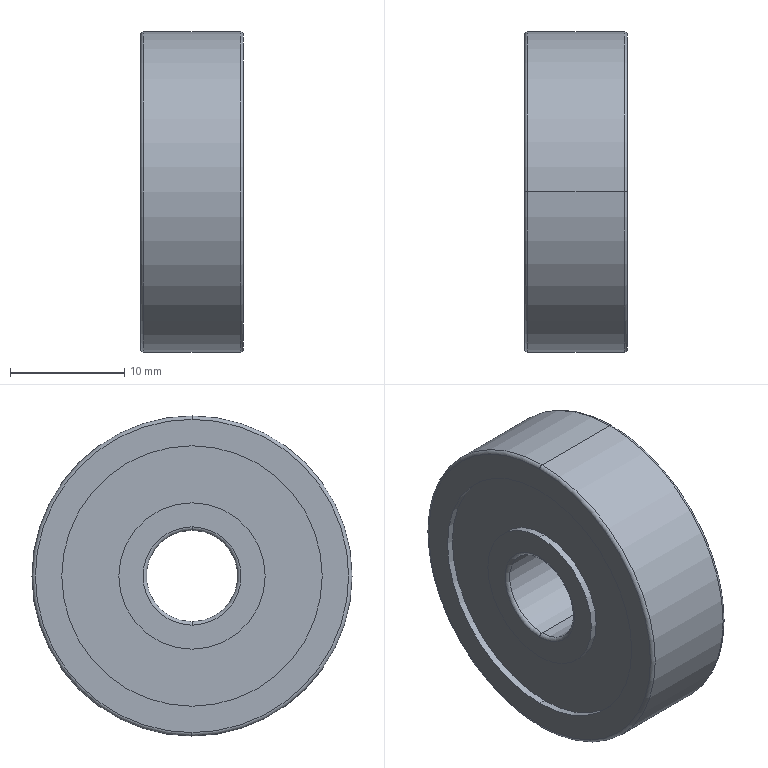Part | SolidWorks | features RefAxis 3, Revolution 1 | 1 solid | 26 faces | box 9 x 28 x 28 mm | volume 4750 mm3 | cylinder 12 | torus 8 | plane 6 | commonest cylinder face diameters 12.8 x4 22.78 x4 8 x2 28 x2
STEP:
#1=CARTESIAN_POINT('',(8.7,0.,-4.));
#2=VERTEX_POINT('',#1);
#3=CARTESIAN_POINT('',(8.7,0.,4.));
#4=VERTEX_POINT('',#3);
#5=CARTESIAN_POINT('',(8.7,0.,0.));
#6=DIRECTION('',(-1.,0.,0.));
#7=DIRECTION('',(0.,0.,1.));
#8=AXIS2_PLACEMENT_3D('',#5,#6,#7);
#9=CIRCLE('',#8,4.);
#10=EDGE_CURVE('',#2,#4,#9,.T.);
#11=ORIENTED_EDGE('',*,*,#10,.F.);
#12=CARTESIAN_POINT('',(0.3,0.,-4.));
#13=VERTEX_POINT('',#12);
#14=CARTESIAN_POINT('',(-0.115,0.,-4.));
#15=DIRECTION('',(-1.,0.,0.));
#16=VECTOR('',#15,1000.);
#17=LINE('',#14,#16);
#18=EDGE_CURVE('',#2,#13,#17,.T.);
#19=ORIENTED_EDGE('',*,*,#18,.T.);
#20=CARTESIAN_POINT('',(0.3,0.,4.));
#21=VERTEX_POINT('',#20);
#22=CARTESIAN_POINT('',(0.3,0.,0.));
#23=DIRECTION('',(-1.,0.,0.));
#24=DIRECTION('',(0.,0.,1.));
#25=AXIS2_PLACEMENT_3D('',#22,#23,#24);
#26=CIRCLE('',#25,4.);
#27=EDGE_CURVE('',#13,#21,#26,.T.);
#28=ORIENTED_EDGE('',*,*,#27,.T.);
#29=CARTESIAN_POINT('',(-0.115,0.,4.));
#30=DIRECTION('',(-1.,0.,0.));
#31=VECTOR('',#30,1000.);
#32=LINE('',#29,#31);
#33=EDGE_CURVE('',#4,#21,#32,.T.);
#34=ORIENTED_EDGE('',*,*,#33,.F.);
#35=EDGE_LOOP('',(#11,#19,#28,#34));
#36=FACE_OUTER_BOUND('',#35,.T.);
#37=CARTESIAN_POINT('',(-0.115,0.,0.));
#38=DIRECTION('',(-1.,0.,0.));
#39=DIRECTION('',(0.,0.,1.));
#40=AXIS2_PLACEMENT_3D('',#37,#38,#39);
#41=CYLINDRICAL_SURFACE('',#40,4.);
#42=ADVANCED_FACE('',(#36),#41,.F.);
#43=CARTESIAN_POINT('',(8.7,0.,0.));
#44=DIRECTION('',(-1.,0.,0.));
#45=DIRECTION('',(0.,0.,1.));
#46=AXIS2_PLACEMENT_3D('',#43,#44,#45);
#47=CIRCLE('',#46,4.);
#48=EDGE_CURVE('',#4,#2,#47,.T.);
#49=ORIENTED_EDGE('',*,*,#48,.T.);
#50=CARTESIAN_POINT('',(9.,0.,-4.3));
#51=VERTEX_POINT('',#50);
#52=CARTESIAN_POINT('',(8.7,0.,-4.3));
#53=DIRECTION('',(0.,1.,0.));
#54=DIRECTION('',(0.,0.,1.));
#55=AXIS2_PLACEMENT_3D('',#52,#53,#54);
#56=CIRCLE('',#55,0.3);
#57=EDGE_CURVE('',#2,#51,#56,.T.);
#58=ORIENTED_EDGE('',*,*,#57,.T.);
#59=CARTESIAN_POINT('',(9.,0.,4.3));
#60=VERTEX_POINT('',#59);
#61=CARTESIAN_POINT('',(9.,0.,0.));
#62=DIRECTION('',(-1.,0.,0.));
#63=DIRECTION('',(0.,0.,1.));
#64=AXIS2_PLACEMENT_3D('',#61,#62,#63);
#65=CIRCLE('',#64,4.3);
#66=EDGE_CURVE('',#60,#51,#65,.T.);
#67=ORIENTED_EDGE('',*,*,#66,.F.);
#68=CARTESIAN_POINT('',(8.7,0.,4.3));
#69=DIRECTION('',(0.,-1.,0.));
#70=DIRECTION('',(0.,0.,-1.));
#71=AXIS2_PLACEMENT_3D('',#68,#69,#70);
#72=CIRCLE('',#71,0.3);
#73=EDGE_CURVE('',#4,#60,#72,.T.);
#74=ORIENTED_EDGE('',*,*,#73,.F.);
#75=EDGE_LOOP('',(#49,#58,#67,#74));
#76=FACE_OUTER_BOUND('',#75,.T.);
#77=CARTESIAN_POINT('',(8.7,0.,0.));
#78=DIRECTION('',(-1.,0.,0.));
#79=DIRECTION('',(0.,0.,1.));
#80=AXIS2_PLACEMENT_3D('',#77,#78,#79);
#81=TOROIDAL_SURFACE('',#80,4.3,0.3);
#82=ADVANCED_FACE('',(#76),#81,.T.);
#83=CARTESIAN_POINT('',(9.,0.,6.4));
#84=VERTEX_POINT('',#83);
#85=CARTESIAN_POINT('',(9.,0.,-6.4));
#86=VERTEX_POINT('',#85);
#87=CARTESIAN_POINT('',(9.,0.,0.));
#88=DIRECTION('',(-1.,0.,0.));
#89=DIRECTION('',(0.,0.,1.));
#90=AXIS2_PLACEMENT_3D('',#87,#88,#89);
#91=CIRCLE('',#90,6.4);
#92=EDGE_CURVE('',#84,#86,#91,.T.);
#93=ORIENTED_EDGE('',*,*,#92,.T.);
#94=CARTESIAN_POINT('',(8.4,0.,-6.4));
#95=VERTEX_POINT('',#94);
#96=CARTESIAN_POINT('',(-0.115,0.,-6.4));
#97=DIRECTION('',(-1.,0.,0.));
#98=VECTOR('',#97,1000.);
#99=LINE('',#96,#98);
#100=EDGE_CURVE('',#86,#95,#99,.T.);
#101=ORIENTED_EDGE('',*,*,#100,.T.);
#102=CARTESIAN_POINT('',(8.4,0.,6.4));
#103=VERTEX_POINT('',#102);
#104=CARTESIAN_POINT('',(8.4,0.,0.));
#105=DIRECTION('',(-1.,0.,0.));
#106=DIRECTION('',(0.,0.,1.));
#107=AXIS2_PLACEMENT_3D('',#104,#105,#106);
#108=CIRCLE('',#107,6.4);
#109=EDGE_CURVE('',#103,#95,#108,.T.);
#110=ORIENTED_EDGE('',*,*,#109,.F.);
#111=CARTESIAN_POINT('',(-0.115,0.,6.4));
#112=DIRECTION('',(-1.,0.,0.));
#113=VECTOR('',#112,1000.);
#114=LINE('',#111,#113);
#115=EDGE_CURVE('',#84,#103,#114,.T.);
#116=ORIENTED_EDGE('',*,*,#115,.F.);
#117=EDGE_LOOP('',(#93,#101,#110,#116));
#118=FACE_OUTER_BOUND('',#117,.T.);
#119=CARTESIAN_POINT('',(-0.115,0.,0.));
#120=DIRECTION('',(-1.,0.,0.));
#121=DIRECTION('',(0.,0.,1.));
#122=AXIS2_PLACEMENT_3D('',#119,#120,#121);
#123=CYLINDRICAL_SURFACE('',#122,6.4);
#124=ADVANCED_FACE('',(#118),#123,.T.);
#125=CARTESIAN_POINT('',(9.,0.,-11.39));
#126=VERTEX_POINT('',#125);
#127=CARTESIAN_POINT('',(9.,0.,11.39));
#128=VERTEX_POINT('',#127);
#129=CARTESIAN_POINT('',(9.,0.,0.));
#130=DIRECTION('',(-1.,0.,0.));
#131=DIRECTION('',(0.,0.,1.));
#132=AXIS2_PLACEMENT_3D('',#129,#130,#131);
#133=CIRCLE('',#132,11.39);
#134=EDGE_CURVE('',#126,#128,#133,.T.);
#135=ORIENTED_EDGE('',*,*,#134,.F.);
#136=CARTESIAN_POINT('',(8.4,0.,-11.39));
#137=VERTEX_POINT('',#136);
#138=CARTESIAN_POINT('',(-0.115,0.,-11.39));
#139=DIRECTION('',(-1.,0.,0.));
#140=VECTOR('',#139,1000.);
#141=LINE('',#138,#140);
#142=EDGE_CURVE('',#126,#137,#141,.T.);
#143=ORIENTED_EDGE('',*,*,#142,.T.);
#144=CARTESIAN_POINT('',(8.4,0.,11.39));
#145=VERTEX_POINT('',#144);
#146=CARTESIAN_POINT('',(8.4,0.,0.));
#147=DIRECTION('',(-1.,0.,0.));
#148=DIRECTION('',(0.,0.,1.));
#149=AXIS2_PLACEMENT_3D('',#146,#147,#148);
#150=CIRCLE('',#149,11.39);
#151=EDGE_CURVE('',#137,#145,#150,.T.);
#152=ORIENTED_EDGE('',*,*,#151,.T.);
#153=CARTESIAN_POINT('',(-0.115,0.,11.39));
#154=DIRECTION('',(-1.,0.,0.));
#155=VECTOR('',#154,1000.);
#156=LINE('',#153,#155);
#157=EDGE_CURVE('',#128,#145,#156,.T.);
#158=ORIENTED_EDGE('',*,*,#157,.F.);
#159=EDGE_LOOP('',(#135,#143,#152,#158));
#160=FACE_OUTER_BOUND('',#159,.T.);
#161=CARTESIAN_POINT('',(-0.115,0.,0.));
#162=DIRECTION('',(-1.,0.,0.));
#163=DIRECTION('',(0.,0.,1.));
#164=AXIS2_PLACEMENT_3D('',#161,#162,#163);
#165=CYLINDRICAL_SURFACE('',#164,11.39);
#166=ADVANCED_FACE('',(#160),#165,.F.);
#167=CARTESIAN_POINT('',(9.,0.,13.7));
#168=VERTEX_POINT('',#167);
#169=CARTESIAN_POINT('',(9.,0.,-13.7));
#170=VERTEX_POINT('',#169);
#171=CARTESIAN_POINT('',(9.,0.,0.));
#172=DIRECTION('',(-1.,0.,0.));
#173=DIRECTION('',(0.,0.,1.));
#174=AXIS2_PLACEMENT_3D('',#171,#172,#173);
#175=CIRCLE('',#174,13.7);
#176=EDGE_CURVE('',#168,#170,#175,.T.);
#177=ORIENTED_EDGE('',*,*,#176,.T.);
#178=CARTESIAN_POINT('',(8.7,0.,-14.));
#179=VERTEX_POINT('',#178);
#180=CARTESIAN_POINT('',(8.7,0.,-13.7));
#181=DIRECTION('',(0.,1.,0.));
#182=DIRECTION('',(0.,0.,1.));
#183=AXIS2_PLACEMENT_3D('',#180,#181,#182);
#184=CIRCLE('',#183,0.3);
#185=EDGE_CURVE('',#170,#179,#184,.T.);
#186=ORIENTED_EDGE('',*,*,#185,.T.);
#187=CARTESIAN_POINT('',(8.7,0.,14.));
#188=VERTEX_POINT('',#187);
#189=CARTESIAN_POINT('',(8.7,0.,0.));
#190=DIRECTION('',(-1.,0.,0.));
#191=DIRECTION('',(0.,0.,1.));
#192=AXIS2_PLACEMENT_3D('',#189,#190,#191);
#193=CIRCLE('',#192,14.);
#194=EDGE_CURVE('',#188,#179,#193,.T.);
#195=ORIENTED_EDGE('',*,*,#194,.F.);
#196=CARTESIAN_POINT('',(8.7,0.,13.7));
#197=DIRECTION('',(0.,-1.,0.));
#198=DIRECTION('',(0.,0.,-1.));
#199=AXIS2_PLACEMENT_3D('',#196,#197,#198);
#200=CIRCLE('',#199,0.3);
#201=EDGE_CURVE('',#168,#188,#200,.T.);
#202=ORIENTED_EDGE('',*,*,#201,.F.);
#203=EDGE_LOOP('',(#177,#186,#195,#202));
#204=FACE_OUTER_BOUND('',#203,.T.);
#205=CARTESIAN_POINT('',(8.7,0.,0.));
#206=DIRECTION('',(-1.,0.,0.));
#207=DIRECTION('',(0.,0.,1.));
#208=AXIS2_PLACEMENT_3D('',#205,#206,#207);
#209=TOROIDAL_SURFACE('',#208,13.7,0.3);
#210=ADVANCED_FACE('',(#204),#209,.T.);
#211=ORIENTED_EDGE('',*,*,#194,.T.);
#212=CARTESIAN_POINT('',(0.3,0.,-14.));
#213=VERTEX_POINT('',#212);
#214=CARTESIAN_POINT('',(-0.115,0.,-14.));
#215=DIRECTION('',(-1.,0.,0.));
#216=VECTOR('',#215,1000.);
#217=LINE('',#214,#216);
#218=EDGE_CURVE('',#179,#213,#217,.T.);
#219=ORIENTED_EDGE('',*,*,#218,.T.);
#220=CARTESIAN_POINT('',(0.3,0.,14.));
#221=VERTEX_POINT('',#220);
#222=CARTESIAN_POINT('',(0.3,0.,0.));
#223=DIRECTION('',(-1.,0.,0.));
#224=DIRECTION('',(0.,0.,1.));
#225=AXIS2_PLACEMENT_3D('',#222,#223,#224);
#226=CIRCLE('',#225,14.);
#227=EDGE_CURVE('',#221,#213,#226,.T.);
#228=ORIENTED_EDGE('',*,*,#227,.F.);
#229=CARTESIAN_POINT('',(-0.115,0.,14.));
#230=DIRECTION('',(-1.,0.,0.));
#231=VECTOR('',#230,1000.);
#232=LINE('',#229,#231);
#233=EDGE_CURVE('',#188,#221,#232,.T.);
#234=ORIENTED_EDGE('',*,*,#233,.F.);
#235=EDGE_LOOP('',(#211,#219,#228,#234));
#236=FACE_OUTER_BOUND('',#235,.T.);
#237=CARTESIAN_POINT('',(-0.115,0.,0.));
#238=DIRECTION('',(-1.,0.,0.));
#239=DIRECTION('',(0.,0.,1.));
#240=AXIS2_PLACEMENT_3D('',#237,#238,#239);
#241=CYLINDRICAL_SURFACE('',#240,14.);
#242=ADVANCED_FACE('',(#236),#241,.T.);
#243=ORIENTED_EDGE('',*,*,#227,.T.);
#244=CARTESIAN_POINT('',(0.,0.,-13.7));
#245=VERTEX_POINT('',#244);
#246=CARTESIAN_POINT('',(0.3,0.,-13.7));
#247=DIRECTION('',(0.,1.,0.));
#248=DIRECTION('',(0.,0.,1.));
#249=AXIS2_PLACEMENT_3D('',#246,#247,#248);
#250=CIRCLE('',#249,0.3);
#251=EDGE_CURVE('',#213,#245,#250,.T.);
#252=ORIENTED_EDGE('',*,*,#251,.T.);
#253=CARTESIAN_POINT('',(0.,0.,13.7));
#254=VERTEX_POINT('',#253);
#255=CARTESIAN_POINT('',(0.,0.,0.));
#256=DIRECTION('',(-1.,0.,0.));
#257=DIRECTION('',(0.,0.,1.));
#258=AXIS2_PLACEMENT_3D('',#255,#256,#257);
#259=CIRCLE('',#258,13.7);
#260=EDGE_CURVE('',#254,#245,#259,.T.);
#261=ORIENTED_EDGE('',*,*,#260,.F.);
#262=CARTESIAN_POINT('',(0.3,0.,13.7));
#263=DIRECTION('',(0.,-1.,0.));
#264=DIRECTION('',(0.,0.,-1.));
#265=AXIS2_PLACEMENT_3D('',#262,#263,#264);
#266=CIRCLE('',#265,0.3);
#267=EDGE_CURVE('',#221,#254,#266,.T.);
#268=ORIENTED_EDGE('',*,*,#267,.F.);
#269=EDGE_LOOP('',(#243,#252,#261,#268));
#270=FACE_OUTER_BOUND('',#269,.T.);
#271=CARTESIAN_POINT('',(0.3,0.,0.));
#272=DIRECTION('',(-1.,0.,0.));
#273=DIRECTION('',(0.,0.,1.));
#274=AXIS2_PLACEMENT_3D('',#271,#272,#273);
#275=TOROIDAL_SURFACE('',#274,13.7,0.3);
#276=ADVANCED_FACE('',(#270),#275,.T.);
#277=CARTESIAN_POINT('',(0.6,0.,-11.39));
#278=VERTEX_POINT('',#277);
#279=CARTESIAN_POINT('',(0.6,0.,11.39));
#280=VERTEX_POINT('',#279);
#281=CARTESIAN_POINT('',(0.6,0.,0.));
#282=DIRECTION('',(-1.,0.,0.));
#283=DIRECTION('',(0.,0.,1.));
#284=AXIS2_PLACEMENT_3D('',#281,#282,#283);
#285=CIRCLE('',#284,11.39);
#286=EDGE_CURVE('',#278,#280,#285,.T.);
#287=ORIENTED_EDGE('',*,*,#286,.F.);
#288=CARTESIAN_POINT('',(0.,0.,-11.39));
#289=VERTEX_POINT('',#288);
#290=CARTESIAN_POINT('',(-0.115,0.,-11.39));
#291=DIRECTION('',(-1.,0.,0.));
#292=VECTOR('',#291,1000.);
#293=LINE('',#290,#292);
#294=EDGE_CURVE('',#278,#289,#293,.T.);
#295=ORIENTED_EDGE('',*,*,#294,.T.);
#296=CARTESIAN_POINT('',(0.,0.,11.39));
#297=VERTEX_POINT('',#296);
#298=CARTESIAN_POINT('',(0.,0.,0.));
#299=DIRECTION('',(-1.,0.,0.));
#300=DIRECTION('',(0.,0.,1.));
#301=AXIS2_PLACEMENT_3D('',#298,#299,#300);
#302=CIRCLE('',#301,11.39);
#303=EDGE_CURVE('',#289,#297,#302,.T.);
#304=ORIENTED_EDGE('',*,*,#303,.T.);
#305=CARTESIAN_POINT('',(-0.115,0.,11.39));
#306=DIRECTION('',(-1.,0.,0.));
#307=VECTOR('',#306,1000.);
#308=LINE('',#305,#307);
#309=EDGE_CURVE('',#280,#297,#308,.T.);
#310=ORIENTED_EDGE('',*,*,#309,.F.);
#311=EDGE_LOOP('',(#287,#295,#304,#310));
#312=FACE_OUTER_BOUND('',#311,.T.);
#313=CARTESIAN_POINT('',(-0.115,0.,0.));
#314=DIRECTION('',(-1.,0.,0.));
#315=DIRECTION('',(0.,0.,1.));
#316=AXIS2_PLACEMENT_3D('',#313,#314,#315);
#317=CYLINDRICAL_SURFACE('',#316,11.39);
#318=ADVANCED_FACE('',(#312),#317,.F.);
#319=CARTESIAN_POINT('',(0.6,0.,6.4));
#320=VERTEX_POINT('',#319);
#321=CARTESIAN_POINT('',(0.6,0.,-6.4));
#322=VERTEX_POINT('',#321);
#323=CARTESIAN_POINT('',(0.6,0.,0.));
#324=DIRECTION('',(-1.,0.,0.));
#325=DIRECTION('',(0.,0.,1.));
#326=AXIS2_PLACEMENT_3D('',#323,#324,#325);
#327=CIRCLE('',#326,6.4);
#328=EDGE_CURVE('',#320,#322,#327,.T.);
#329=ORIENTED_EDGE('',*,*,#328,.T.);
#330=CARTESIAN_POINT('',(0.,0.,-6.4));
#331=VERTEX_POINT('',#330);
#332=CARTESIAN_POINT('',(-0.115,0.,-6.4));
#333=DIRECTION('',(-1.,0.,0.));
#334=VECTOR('',#333,1000.);
#335=LINE('',#332,#334);
#336=EDGE_CURVE('',#322,#331,#335,.T.);
#337=ORIENTED_EDGE('',*,*,#336,.T.);
#338=CARTESIAN_POINT('',(0.,0.,6.4));
#339=VERTEX_POINT('',#338);
#340=CARTESIAN_POINT('',(0.,0.,0.));
#341=DIRECTION('',(-1.,0.,0.));
#342=DIRECTION('',(0.,0.,1.));
#343=AXIS2_PLACEMENT_3D('',#340,#341,#342);
#344=CIRCLE('',#343,6.4);
#345=EDGE_CURVE('',#339,#331,#344,.T.);
#346=ORIENTED_EDGE('',*,*,#345,.F.);
#347=CARTESIAN_POINT('',(-0.115,0.,6.4));
#348=DIRECTION('',(-1.,0.,0.));
#349=VECTOR('',#348,1000.);
#350=LINE('',#347,#349);
#351=EDGE_CURVE('',#320,#339,#350,.T.);
#352=ORIENTED_EDGE('',*,*,#351,.F.);
#353=EDGE_LOOP('',(#329,#337,#346,#352));
#354=FACE_OUTER_BOUND('',#353,.T.);
#355=CARTESIAN_POINT('',(-0.115,0.,0.));
#356=DIRECTION('',(-1.,0.,0.));
#357=DIRECTION('',(0.,0.,1.));
#358=AXIS2_PLACEMENT_3D('',#355,#356,#357);
#359=CYLINDRICAL_SURFACE('',#358,6.4);
#360=ADVANCED_FACE('',(#354),#359,.T.);
#361=CARTESIAN_POINT('',(0.,0.,4.3));
#362=VERTEX_POINT('',#361);
#363=CARTESIAN_POINT('',(0.,0.,-4.3));
#364=VERTEX_POINT('',#363);
#365=CARTESIAN_POINT('',(0.,0.,0.));
#366=DIRECTION('',(-1.,0.,0.));
#367=DIRECTION('',(0.,0.,1.));
#368=AXIS2_PLACEMENT_3D('',#365,#366,#367);
#369=CIRCLE('',#368,4.3);
#370=EDGE_CURVE('',#362,#364,#369,.T.);
#371=ORIENTED_EDGE('',*,*,#370,.T.);
#372=CARTESIAN_POINT('',(0.3,0.,-4.3));
#373=DIRECTION('',(0.,1.,0.));
#374=DIRECTION('',(0.,0.,1.));
#375=AXIS2_PLACEMENT_3D('',#372,#373,#374);
#376=CIRCLE('',#375,0.3);
#377=EDGE_CURVE('',#364,#13,#376,.T.);
#378=ORIENTED_EDGE('',*,*,#377,.T.);
#379=CARTESIAN_POINT('',(0.3,0.,0.));
#380=DIRECTION('',(-1.,0.,0.));
#381=DIRECTION('',(0.,0.,1.));
#382=AXIS2_PLACEMENT_3D('',#379,#380,#381);
#383=CIRCLE('',#382,4.);
#384=EDGE_CURVE('',#21,#13,#383,.T.);
#385=ORIENTED_EDGE('',*,*,#384,.F.);
#386=CARTESIAN_POINT('',(0.3,0.,4.3));
#387=DIRECTION('',(0.,-1.,0.));
#388=DIRECTION('',(0.,0.,-1.));
#389=AXIS2_PLACEMENT_3D('',#386,#387,#388);
#390=CIRCLE('',#389,0.3);
#391=EDGE_CURVE('',#362,#21,#390,.T.);
#392=ORIENTED_EDGE('',*,*,#391,.F.);
#393=EDGE_LOOP('',(#371,#378,#385,#392));
#394=FACE_OUTER_BOUND('',#393,.T.);
#395=CARTESIAN_POINT('',(0.3,0.,0.));
#396=DIRECTION('',(-1.,0.,0.));
#397=DIRECTION('',(0.,0.,1.));
#398=AXIS2_PLACEMENT_3D('',#395,#396,#397);
#399=TOROIDAL_SURFACE('',#398,4.3,0.3);
#400=ADVANCED_FACE('',(#394),#399,.T.);
#401=ORIENTED_EDGE('',*,*,#377,.F.);
#402=CARTESIAN_POINT('',(0.,0.,0.));
#403=DIRECTION('',(-1.,0.,0.));
#404=DIRECTION('',(0.,0.,1.));
#405=AXIS2_PLACEMENT_3D('',#402,#403,#404);
#406=CIRCLE('',#405,4.3);
#407=EDGE_CURVE('',#364,#362,#406,.T.);
#408=ORIENTED_EDGE('',*,*,#407,.T.);
#409=ORIENTED_EDGE('',*,*,#391,.T.);
#410=ORIENTED_EDGE('',*,*,#27,.F.);
#411=EDGE_LOOP('',(#401,#408,#409,#410));
#412=FACE_OUTER_BOUND('',#411,.T.);
#413=CARTESIAN_POINT('',(0.3,0.,0.));
#414=DIRECTION('',(-1.,0.,0.));
#415=DIRECTION('',(0.,0.,1.));
#416=AXIS2_PLACEMENT_3D('',#413,#414,#415);
#417=TOROIDAL_SURFACE('',#416,4.3,0.3);
#418=ADVANCED_FACE('',(#412),#417,.T.);
#419=ORIENTED_EDGE('',*,*,#370,.F.);
#420=ORIENTED_EDGE('',*,*,#407,.F.);
#421=EDGE_LOOP('',(#419,#420));
#422=FACE_BOUND('',#421,.T.);
#423=ORIENTED_EDGE('',*,*,#345,.T.);
#424=CARTESIAN_POINT('',(0.,0.,0.));
#425=DIRECTION('',(-1.,0.,0.));
#426=DIRECTION('',(0.,0.,1.));
#427=AXIS2_PLACEMENT_3D('',#424,#425,#426);
#428=CIRCLE('',#427,6.4);
#429=EDGE_CURVE('',#331,#339,#428,.T.);
#430=ORIENTED_EDGE('',*,*,#429,.T.);
#431=EDGE_LOOP('',(#423,#430));
#432=FACE_OUTER_BOUND('',#431,.T.);
#433=CARTESIAN_POINT('',(0.,6.4,0.));
#434=DIRECTION('',(1.,0.,0.));
#435=DIRECTION('',(0.,0.,-1.));
#436=AXIS2_PLACEMENT_3D('',#433,#434,#435);
#437=PLANE('',#436);
#438=ADVANCED_FACE('',(#422,#432),#437,.F.);
#439=ORIENTED_EDGE('',*,*,#336,.F.);
#440=CARTESIAN_POINT('',(0.6,0.,0.));
#441=DIRECTION('',(-1.,0.,0.));
#442=DIRECTION('',(0.,0.,1.));
#443=AXIS2_PLACEMENT_3D('',#440,#441,#442);
#444=CIRCLE('',#443,6.4);
#445=EDGE_CURVE('',#322,#320,#444,.T.);
#446=ORIENTED_EDGE('',*,*,#445,.T.);
#447=ORIENTED_EDGE('',*,*,#351,.T.);
#448=ORIENTED_EDGE('',*,*,#429,.F.);
#449=EDGE_LOOP('',(#439,#446,#447,#448));
#450=FACE_OUTER_BOUND('',#449,.T.);
#451=CARTESIAN_POINT('',(-0.115,0.,0.));
#452=DIRECTION('',(-1.,0.,0.));
#453=DIRECTION('',(0.,0.,1.));
#454=AXIS2_PLACEMENT_3D('',#451,#452,#453);
#455=CYLINDRICAL_SURFACE('',#454,6.4);
#456=ADVANCED_FACE('',(#450),#455,.T.);
#457=ORIENTED_EDGE('',*,*,#328,.F.);
#458=ORIENTED_EDGE('',*,*,#445,.F.);
#459=EDGE_LOOP('',(#457,#458));
#460=FACE_BOUND('',#459,.T.);
#461=CARTESIAN_POINT('',(0.6,0.,0.));
#462=DIRECTION('',(-1.,0.,0.));
#463=DIRECTION('',(0.,0.,1.));
#464=AXIS2_PLACEMENT_3D('',#461,#462,#463);
#465=CIRCLE('',#464,11.39);
#466=EDGE_CURVE('',#280,#278,#465,.T.);
#467=ORIENTED_EDGE('',*,*,#466,.T.);
#468=ORIENTED_EDGE('',*,*,#286,.T.);
#469=EDGE_LOOP('',(#467,#468));
#470=FACE_OUTER_BOUND('',#469,.T.);
#471=CARTESIAN_POINT('',(0.6,11.39,0.));
#472=DIRECTION('',(1.,0.,0.));
#473=DIRECTION('',(0.,0.,-1.));
#474=AXIS2_PLACEMENT_3D('',#471,#472,#473);
#475=PLANE('',#474);
#476=ADVANCED_FACE('',(#460,#470),#475,.F.);
#477=ORIENTED_EDGE('',*,*,#294,.F.);
#478=ORIENTED_EDGE('',*,*,#466,.F.);
#479=ORIENTED_EDGE('',*,*,#309,.T.);
#480=CARTESIAN_POINT('',(0.,0.,0.));
#481=DIRECTION('',(-1.,0.,0.));
#482=DIRECTION('',(0.,0.,1.));
#483=AXIS2_PLACEMENT_3D('',#480,#481,#482);
#484=CIRCLE('',#483,11.39);
#485=EDGE_CURVE('',#297,#289,#484,.T.);
#486=ORIENTED_EDGE('',*,*,#485,.T.);
#487=EDGE_LOOP('',(#477,#478,#479,#486));
#488=FACE_OUTER_BOUND('',#487,.T.);
#489=CARTESIAN_POINT('',(-0.115,0.,0.));
#490=DIRECTION('',(-1.,0.,0.));
#491=DIRECTION('',(0.,0.,1.));
#492=AXIS2_PLACEMENT_3D('',#489,#490,#491);
#493=CYLINDRICAL_SURFACE('',#492,11.39);
#494=ADVANCED_FACE('',(#488),#493,.F.);
#495=ORIENTED_EDGE('',*,*,#485,.F.);
#496=ORIENTED_EDGE('',*,*,#303,.F.);
#497=EDGE_LOOP('',(#495,#496));
#498=FACE_BOUND('',#497,.T.);
#499=ORIENTED_EDGE('',*,*,#260,.T.);
#500=CARTESIAN_POINT('',(0.,0.,0.));
#501=DIRECTION('',(-1.,0.,0.));
#502=DIRECTION('',(0.,0.,1.));
#503=AXIS2_PLACEMENT_3D('',#500,#501,#502);
#504=CIRCLE('',#503,13.7);
#505=EDGE_CURVE('',#245,#254,#504,.T.);
#506=ORIENTED_EDGE('',*,*,#505,.T.);
#507=EDGE_LOOP('',(#499,#506));
#508=FACE_OUTER_BOUND('',#507,.T.);
#509=CARTESIAN_POINT('',(0.,13.7,0.));
#510=DIRECTION('',(1.,0.,0.));
#511=DIRECTION('',(0.,0.,-1.));
#512=AXIS2_PLACEMENT_3D('',#509,#510,#511);
#513=PLANE('',#512);
#514=ADVANCED_FACE('',(#498,#508),#513,.F.);
#515=ORIENTED_EDGE('',*,*,#251,.F.);
#516=CARTESIAN_POINT('',(0.3,0.,0.));
#517=DIRECTION('',(-1.,0.,0.));
#518=DIRECTION('',(0.,0.,1.));
#519=AXIS2_PLACEMENT_3D('',#516,#517,#518);
#520=CIRCLE('',#519,14.);
#521=EDGE_CURVE('',#213,#221,#520,.T.);
#522=ORIENTED_EDGE('',*,*,#521,.T.);
#523=ORIENTED_EDGE('',*,*,#267,.T.);
#524=ORIENTED_EDGE('',*,*,#505,.F.);
#525=EDGE_LOOP('',(#515,#522,#523,#524));
#526=FACE_OUTER_BOUND('',#525,.T.);
#527=CARTESIAN_POINT('',(0.3,0.,0.));
#528=DIRECTION('',(-1.,0.,0.));
#529=DIRECTION('',(0.,0.,1.));
#530=AXIS2_PLACEMENT_3D('',#527,#528,#529);
#531=TOROIDAL_SURFACE('',#530,13.7,0.3);
#532=ADVANCED_FACE('',(#526),#531,.T.);
#533=ORIENTED_EDGE('',*,*,#218,.F.);
#534=CARTESIAN_POINT('',(8.7,0.,0.));
#535=DIRECTION('',(-1.,0.,0.));
#536=DIRECTION('',(0.,0.,1.));
#537=AXIS2_PLACEMENT_3D('',#534,#535,#536);
#538=CIRCLE('',#537,14.);
#539=EDGE_CURVE('',#179,#188,#538,.T.);
#540=ORIENTED_EDGE('',*,*,#539,.T.);
#541=ORIENTED_EDGE('',*,*,#233,.T.);
#542=ORIENTED_EDGE('',*,*,#521,.F.);
#543=EDGE_LOOP('',(#533,#540,#541,#542));
#544=FACE_OUTER_BOUND('',#543,.T.);
#545=CARTESIAN_POINT('',(-0.115,0.,0.));
#546=DIRECTION('',(-1.,0.,0.));
#547=DIRECTION('',(0.,0.,1.));
#548=AXIS2_PLACEMENT_3D('',#545,#546,#547);
#549=CYLINDRICAL_SURFACE('',#548,14.);
#550=ADVANCED_FACE('',(#544),#549,.T.);
#551=ORIENTED_EDGE('',*,*,#185,.F.);
#552=CARTESIAN_POINT('',(9.,0.,0.));
#553=DIRECTION('',(-1.,0.,0.));
#554=DIRECTION('',(0.,0.,1.));
#555=AXIS2_PLACEMENT_3D('',#552,#553,#554);
#556=CIRCLE('',#555,13.7);
#557=EDGE_CURVE('',#170,#168,#556,.T.);
#558=ORIENTED_EDGE('',*,*,#557,.T.);
#559=ORIENTED_EDGE('',*,*,#201,.T.);
#560=ORIENTED_EDGE('',*,*,#539,.F.);
#561=EDGE_LOOP('',(#551,#558,#559,#560));
#562=FACE_OUTER_BOUND('',#561,.T.);
#563=CARTESIAN_POINT('',(8.7,0.,0.));
#564=DIRECTION('',(-1.,0.,0.));
#565=DIRECTION('',(0.,0.,1.));
#566=AXIS2_PLACEMENT_3D('',#563,#564,#565);
#567=TOROIDAL_SURFACE('',#566,13.7,0.3);
#568=ADVANCED_FACE('',(#562),#567,.T.);
#569=ORIENTED_EDGE('',*,*,#176,.F.);
#570=ORIENTED_EDGE('',*,*,#557,.F.);
#571=EDGE_LOOP('',(#569,#570));
#572=FACE_OUTER_BOUND('',#571,.T.);
#573=CARTESIAN_POINT('',(9.,0.,0.));
#574=DIRECTION('',(-1.,0.,0.));
#575=DIRECTION('',(0.,0.,1.));
#576=AXIS2_PLACEMENT_3D('',#573,#574,#575);
#577=CIRCLE('',#576,11.39);
#578=EDGE_CURVE('',#128,#126,#577,.T.);
#579=ORIENTED_EDGE('',*,*,#578,.T.);
#580=ORIENTED_EDGE('',*,*,#134,.T.);
#581=EDGE_LOOP('',(#579,#580));
#582=FACE_BOUND('',#581,.T.);
#583=CARTESIAN_POINT('',(9.,13.7,0.));
#584=DIRECTION('',(-1.,0.,0.));
#585=DIRECTION('',(0.,0.,1.));
#586=AXIS2_PLACEMENT_3D('',#583,#584,#585);
#587=PLANE('',#586);
#588=ADVANCED_FACE('',(#572,#582),#587,.F.);
#589=ORIENTED_EDGE('',*,*,#142,.F.);
#590=ORIENTED_EDGE('',*,*,#578,.F.);
#591=ORIENTED_EDGE('',*,*,#157,.T.);
#592=CARTESIAN_POINT('',(8.4,0.,0.));
#593=DIRECTION('',(-1.,0.,0.));
#594=DIRECTION('',(0.,0.,1.));
#595=AXIS2_PLACEMENT_3D('',#592,#593,#594);
#596=CIRCLE('',#595,11.39);
#597=EDGE_CURVE('',#145,#137,#596,.T.);
#598=ORIENTED_EDGE('',*,*,#597,.T.);
#599=EDGE_LOOP('',(#589,#590,#591,#598));
#600=FACE_OUTER_BOUND('',#599,.T.);
#601=CARTESIAN_POINT('',(-0.115,0.,0.));
#602=DIRECTION('',(-1.,0.,0.));
#603=DIRECTION('',(0.,0.,1.));
#604=AXIS2_PLACEMENT_3D('',#601,#602,#603);
#605=CYLINDRICAL_SURFACE('',#604,11.39);
#606=ADVANCED_FACE('',(#600),#605,.F.);
#607=ORIENTED_EDGE('',*,*,#597,.F.);
#608=ORIENTED_EDGE('',*,*,#151,.F.);
#609=EDGE_LOOP('',(#607,#608));
#610=FACE_OUTER_BOUND('',#609,.T.);
#611=ORIENTED_EDGE('',*,*,#109,.T.);
#612=CARTESIAN_POINT('',(8.4,0.,0.));
#613=DIRECTION('',(-1.,0.,0.));
#614=DIRECTION('',(0.,0.,1.));
#615=AXIS2_PLACEMENT_3D('',#612,#613,#614);
#616=CIRCLE('',#615,6.4);
#617=EDGE_CURVE('',#95,#103,#616,.T.);
#618=ORIENTED_EDGE('',*,*,#617,.T.);
#619=EDGE_LOOP('',(#611,#618));
#620=FACE_BOUND('',#619,.T.);
#621=CARTESIAN_POINT('',(8.4,11.39,0.));
#622=DIRECTION('',(-1.,0.,0.));
#623=DIRECTION('',(0.,0.,1.));
#624=AXIS2_PLACEMENT_3D('',#621,#622,#623);
#625=PLANE('',#624);
#626=ADVANCED_FACE('',(#610,#620),#625,.F.);
#627=ORIENTED_EDGE('',*,*,#100,.F.);
#628=CARTESIAN_POINT('',(9.,0.,0.));
#629=DIRECTION('',(-1.,0.,0.));
#630=DIRECTION('',(0.,0.,1.));
#631=AXIS2_PLACEMENT_3D('',#628,#629,#630);
#632=CIRCLE('',#631,6.4);
#633=EDGE_CURVE('',#86,#84,#632,.T.);
#634=ORIENTED_EDGE('',*,*,#633,.T.);
#635=ORIENTED_EDGE('',*,*,#115,.T.);
#636=ORIENTED_EDGE('',*,*,#617,.F.);
#637=EDGE_LOOP('',(#627,#634,#635,#636));
#638=FACE_OUTER_BOUND('',#637,.T.);
#639=CARTESIAN_POINT('',(-0.115,0.,0.));
#640=DIRECTION('',(-1.,0.,0.));
#641=DIRECTION('',(0.,0.,1.));
#642=AXIS2_PLACEMENT_3D('',#639,#640,#641);
#643=CYLINDRICAL_SURFACE('',#642,6.4);
#644=ADVANCED_FACE('',(#638),#643,.T.);
#645=ORIENTED_EDGE('',*,*,#92,.F.);
#646=ORIENTED_EDGE('',*,*,#633,.F.);
#647=EDGE_LOOP('',(#645,#646));
#648=FACE_OUTER_BOUND('',#647,.T.);
#649=ORIENTED_EDGE('',*,*,#66,.T.);
#650=CARTESIAN_POINT('',(9.,0.,0.));
#651=DIRECTION('',(-1.,0.,0.));
#652=DIRECTION('',(0.,0.,1.));
#653=AXIS2_PLACEMENT_3D('',#650,#651,#652);
#654=CIRCLE('',#653,4.3);
#655=EDGE_CURVE('',#51,#60,#654,.T.);
#656=ORIENTED_EDGE('',*,*,#655,.T.);
#657=EDGE_LOOP('',(#649,#656));
#658=FACE_BOUND('',#657,.T.);
#659=CARTESIAN_POINT('',(9.,6.4,0.));
#660=DIRECTION('',(-1.,0.,0.));
#661=DIRECTION('',(0.,0.,1.));
#662=AXIS2_PLACEMENT_3D('',#659,#660,#661);
#663=PLANE('',#662);
#664=ADVANCED_FACE('',(#648,#658),#663,.F.);
#665=ORIENTED_EDGE('',*,*,#57,.F.);
#666=ORIENTED_EDGE('',*,*,#10,.T.);
#667=ORIENTED_EDGE('',*,*,#73,.T.);
#668=ORIENTED_EDGE('',*,*,#655,.F.);
#669=EDGE_LOOP('',(#665,#666,#667,#668));
#670=FACE_OUTER_BOUND('',#669,.T.);
#671=CARTESIAN_POINT('',(8.7,0.,0.));
#672=DIRECTION('',(-1.,0.,0.));
#673=DIRECTION('',(0.,0.,1.));
#674=AXIS2_PLACEMENT_3D('',#671,#672,#673);
#675=TOROIDAL_SURFACE('',#674,4.3,0.3);
#676=ADVANCED_FACE('',(#670),#675,.T.);
#677=ORIENTED_EDGE('',*,*,#18,.F.);
#678=ORIENTED_EDGE('',*,*,#48,.F.);
#679=ORIENTED_EDGE('',*,*,#33,.T.);
#680=ORIENTED_EDGE('',*,*,#384,.T.);
#681=EDGE_LOOP('',(#677,#678,#679,#680));
#682=FACE_OUTER_BOUND('',#681,.T.);
#683=CARTESIAN_POINT('',(-0.115,0.,0.));
#684=DIRECTION('',(-1.,0.,0.));
#685=DIRECTION('',(0.,0.,1.));
#686=AXIS2_PLACEMENT_3D('',#683,#684,#685);
#687=CYLINDRICAL_SURFACE('',#686,4.);
#688=ADVANCED_FACE('',(#682),#687,.F.);
#689=CLOSED_SHELL('',(#42,#82,#124,#166,#210,#242,#276,#318,#360,#400,#418,#438,#456,#476,#494,#514,#532,#550,#568,#588,#606,#626,#644,#664,#676,#688));
#690=MANIFOLD_SOLID_BREP('',#689);
#691=CARTESIAN_POINT('',(0.,0.,0.));
#692=DIRECTION('',(0.,0.,1.));
#693=DIRECTION('',(1.,0.,0.));
#694=AXIS2_PLACEMENT_3D('',#691,#692,#693);
#695=(LENGTH_UNIT()NAMED_UNIT(*)SI_UNIT(.MILLI.,.METRE.));
#696=UNCERTAINTY_MEASURE_WITH_UNIT(LENGTH_MEASURE(0.00001),#695,'','');
#697=(NAMED_UNIT(*)PLANE_ANGLE_UNIT()SI_UNIT($,.RADIAN.));
#698=(NAMED_UNIT(*)SI_UNIT($,.STERADIAN.)SOLID_ANGLE_UNIT());
#699=(GEOMETRIC_REPRESENTATION_CONTEXT(3)GLOBAL_UNCERTAINTY_ASSIGNED_CONTEXT((#696))GLOBAL_UNIT_ASSIGNED_CONTEXT((#695,#697,#698))REPRESENTATION_CONTEXT('',''));
#700=ADVANCED_BREP_SHAPE_REPRESENTATION('',(#690,#694),#699);